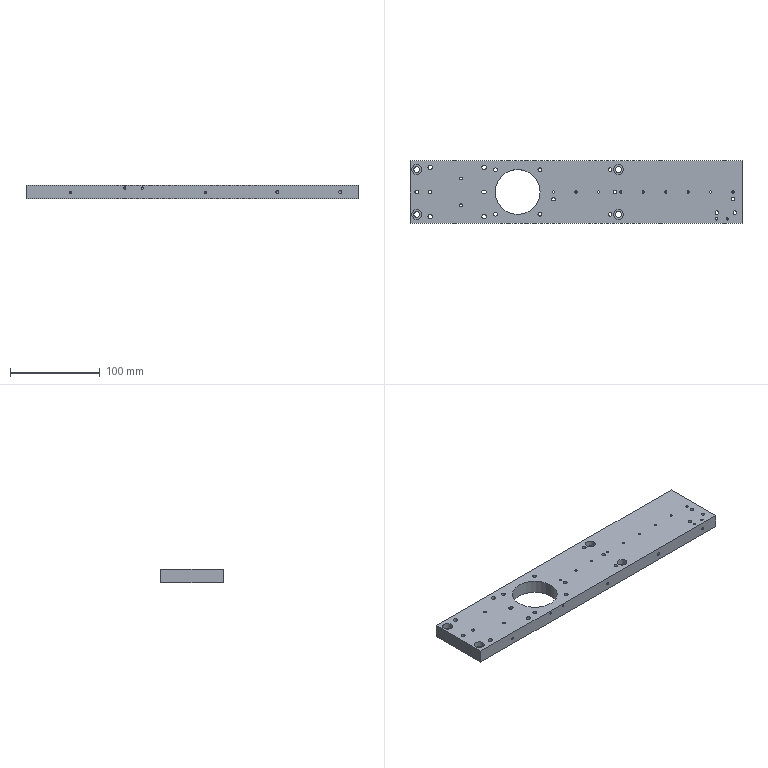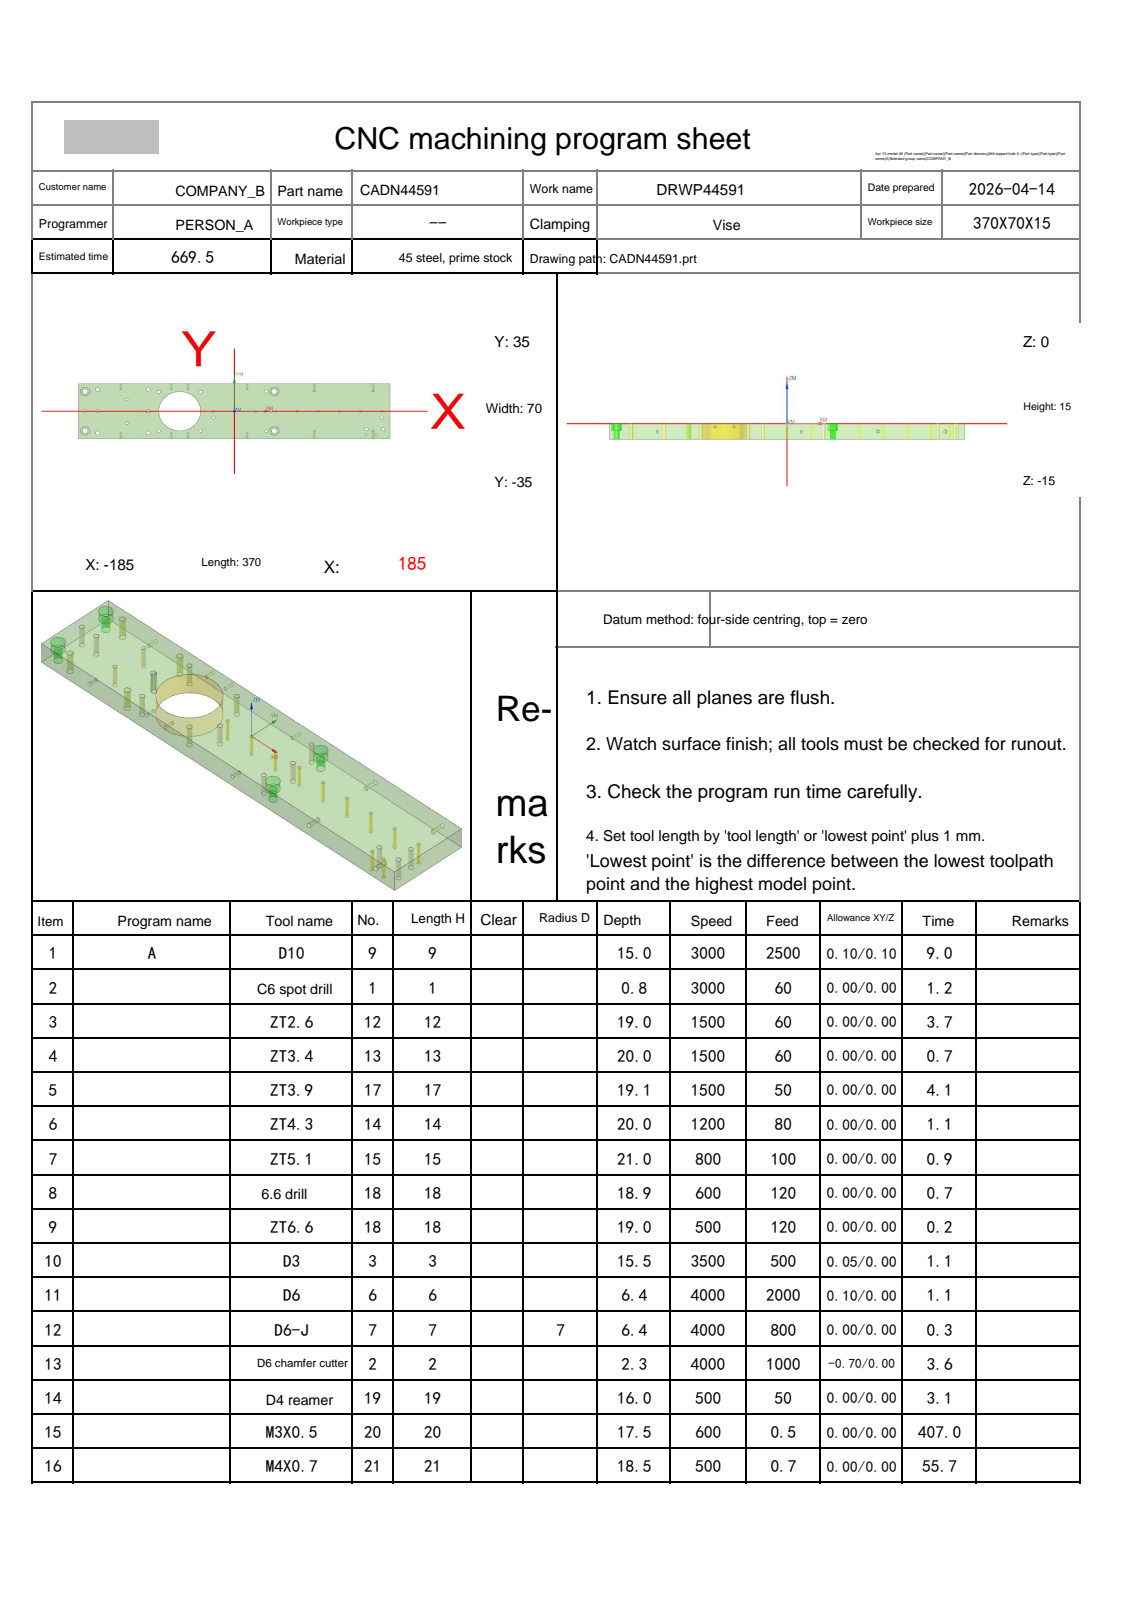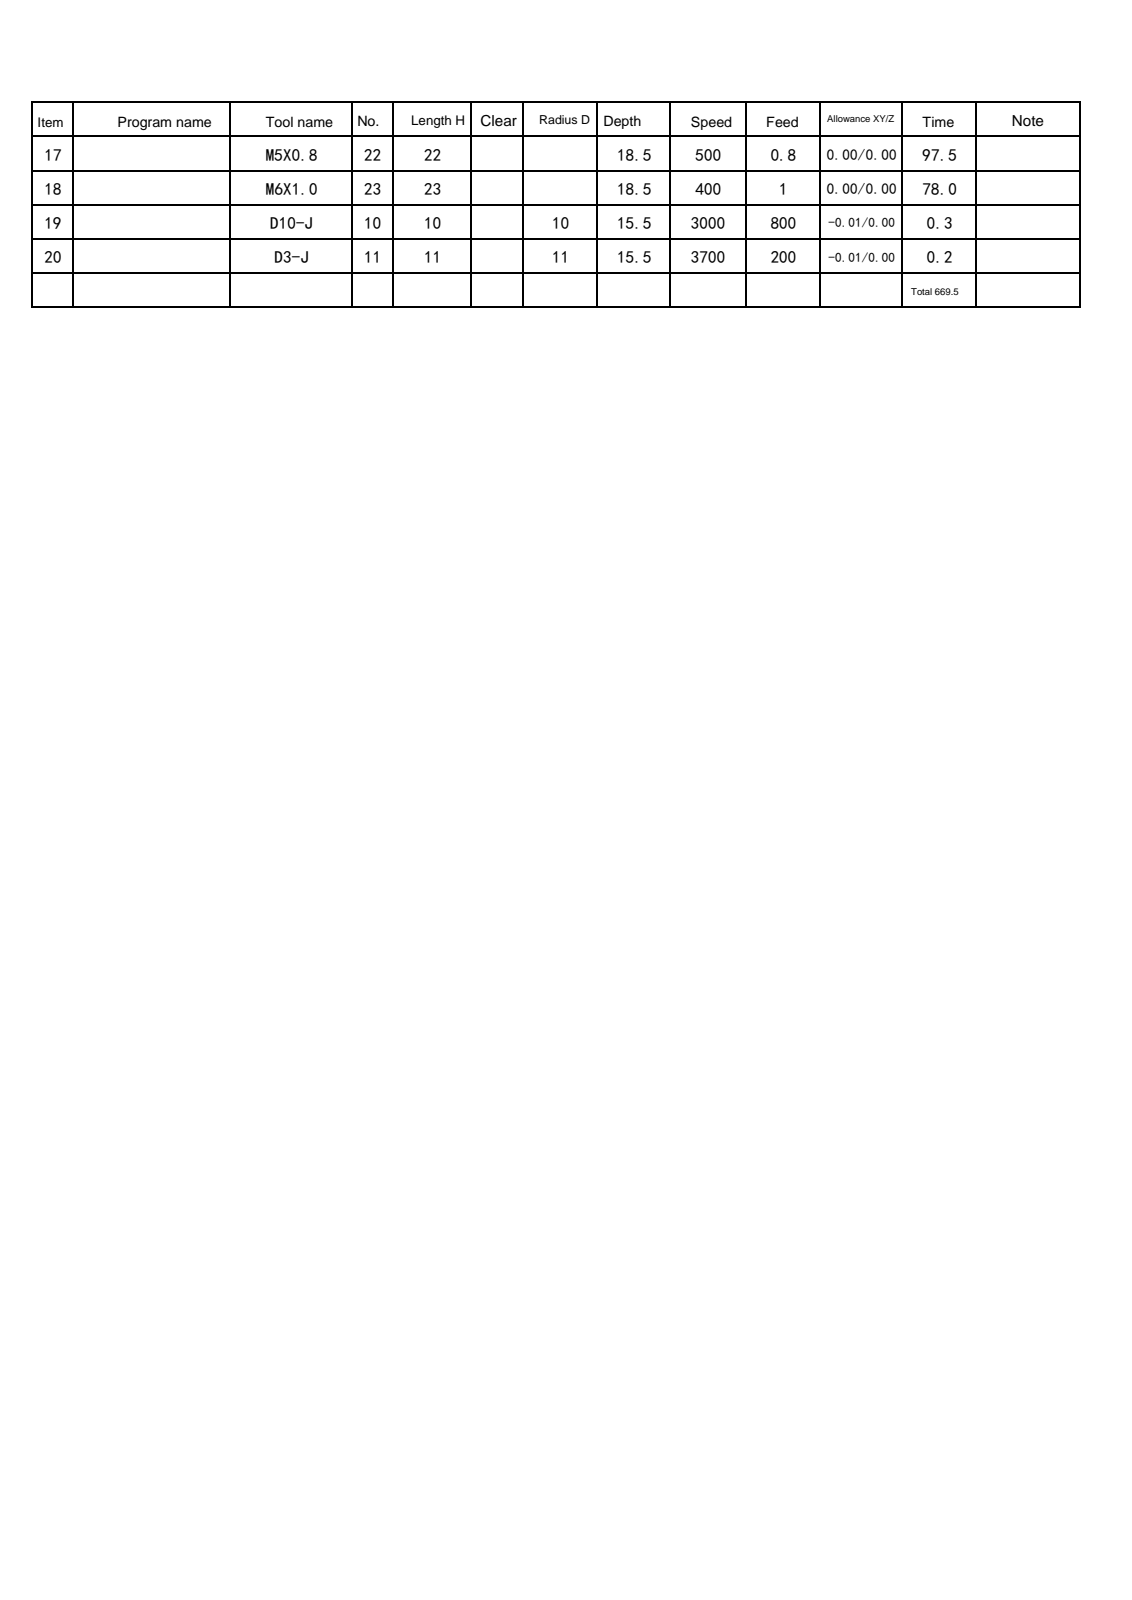NC program | NX | posted by the shop | part box 370 x 70 x 15 mm
Lines 1 to 28 of 4500:
%
O0001
(Machine time: 1277.78 MIN)
(===Total Tool:19===)
(T9=D10     D=10.  R=0.   D-  H09 Z=-15.  )
(T1=C6 spot drill   D=6.   R=0.   D-  H01 Z=-0.8  )
(T12=ZT2.6  D=2.6  DR_a=118 D-  H12 Z=-19.  )
(T13=ZT3.4  D=3.4  DR_a=118 D-  H13 Z=-20.  )
(T17=ZT3.9  D=3.9  DR_a=120 D-  H17 Z=-19.13)
(T14=ZT4.3  D=4.3  DR_a=118 D-  H14 Z=-20.  )
(T15=ZT5.1  D=5.1  DR_a=118 D-  H15 Z=-21.  )
(T18=6.6 drill  D=6.6  DR_a=120 D-  H18 Z=-18.98)
(T3=D3      D=3.   R=0.   D-  H03 Z=-15.5 )
(T6=D6      D=6.   R=0.   D-  H06 Z=-6.4  )
(T7=D6-J    D=6.   R=0.   D7  H07 Z=-6.4  )
(T2=D6 chamfer cutter   D=6.   R=0.   D-  H02 Z=-2.3  )
(T19=D4 reamer   D=4.   DR_a=180 D-  H19 Z=-16.  )
(T20=M3X0.5 D=2.5  DR_a=180 D-  H20 Z=-17.5 )
(T21=M4X0.7 D=3.3  DR_a=180 D-  H21 Z=-18.5 )
(T22=M5X0.8 D=4.2  DR_a=180 D-  H22 Z=-18.5 )
(T23=M6X1.0 D=5.   DR_a=180 D-  H23 Z=-18.5 )
(T10=D10-J  D=10.  R=0.   D10 H10 Z=-15.5 )
(T11=D3-J   D=3.   R=0.   D11 H11 Z=-15.5 )
G80 G90 G17 G49 G40
G91 G28 Z0
M01